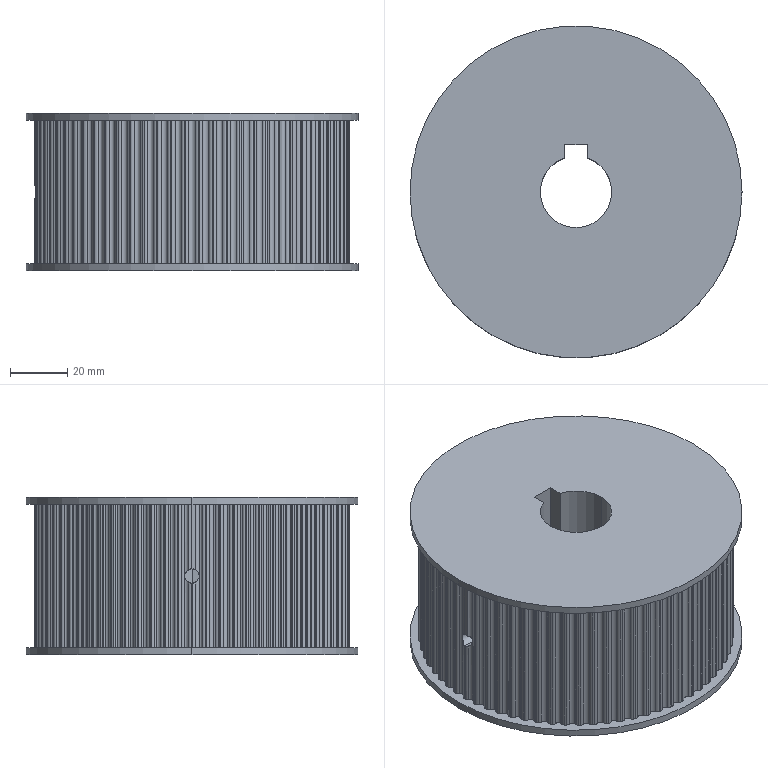Part | 1 solid | 348 faces | box 116 x 116 x 55 mm | volume 488123 mm3 | cylinder 341 | plane 7 | commonest cylinder face diameters 2.5 x257 110 x73 5 x4 116 x4 25 x3